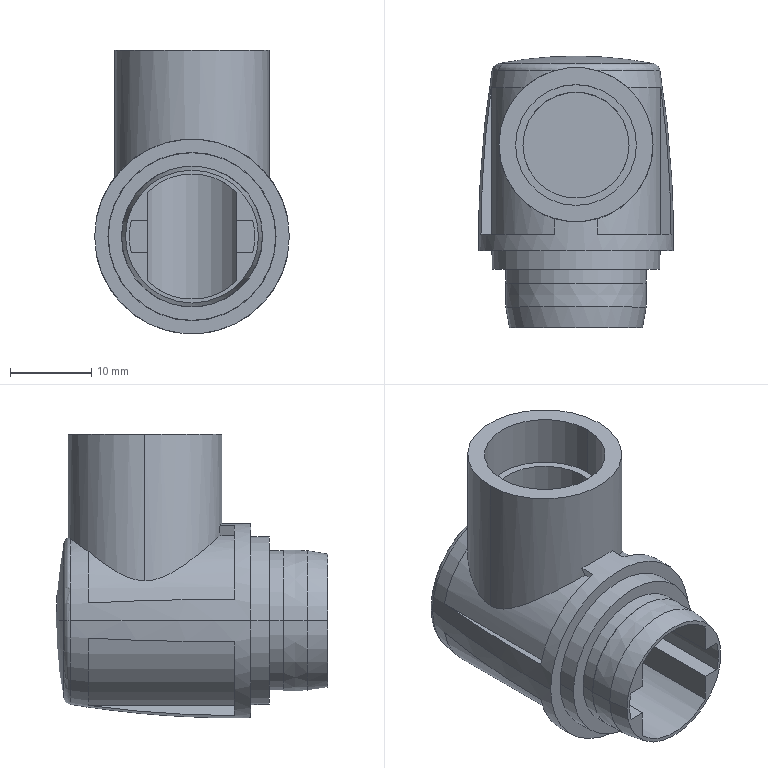Part | STEP file | 2023_07_21_12_39_19_0129 | 1 solid | 57 faces | box 24.025 x 33.5 x 35.012 mm | volume 7738 mm3 | plane 29 | cylinder 16 | cone 6 | spline 2 | sphere 2 | torus 2 | commonest cylinder face diameters 15.5 x4 21.371 x4 13.1 x2 14.9 x2 17.3 x2 19 x2